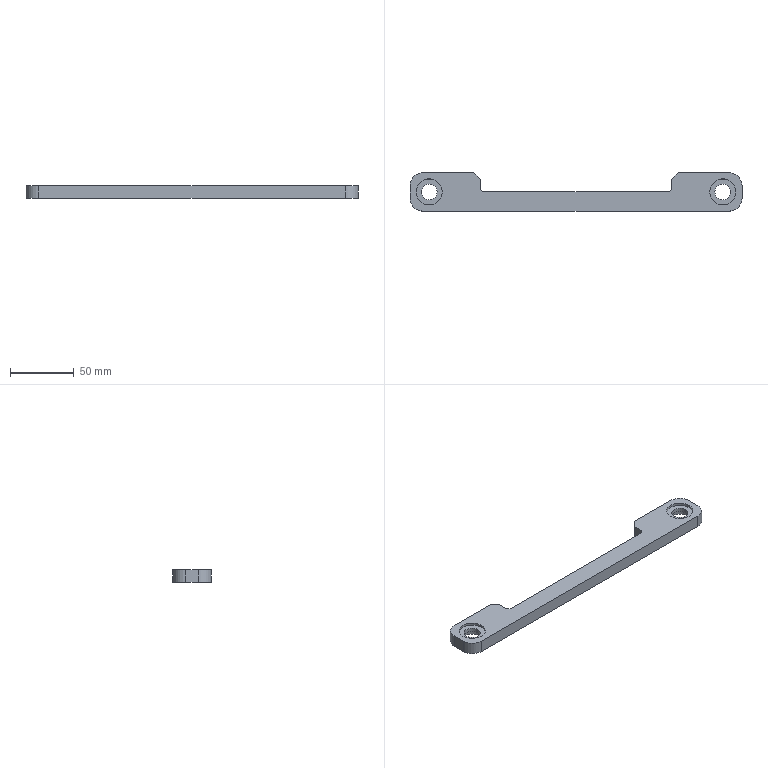Part | SolidWorks | features BaseBody 1 | 1 solid | 34 faces | box 260 x 30 x 10 mm | volume 49540 mm3 | plane 18 | cylinder 16 | commonest cylinder face diameters 12.5 x4 19 x4 20 x4 20.5 x4
STEP:
#1=CARTESIAN_POINT('',(-105.5,-44.517,281.481));
#2=VERTEX_POINT('',#1);
#3=CARTESIAN_POINT('',(-124.5,-44.517,281.481));
#4=VERTEX_POINT('',#3);
#5=CARTESIAN_POINT('',(-115.,-44.517,281.481));
#6=DIRECTION('',(0.,0.,-1.));
#7=DIRECTION('',(-1.,0.,0.));
#8=AXIS2_PLACEMENT_3D('',#5,#6,#7);
#9=CIRCLE('',#8,9.5);
#10=EDGE_CURVE('',#2,#4,#9,.T.);
#11=ORIENTED_EDGE('',*,*,#10,.F.);
#12=CARTESIAN_POINT('',(-105.5,-44.517,276.481));
#13=VERTEX_POINT('',#12);
#14=CARTESIAN_POINT('',(-105.5,-44.517,281.481));
#15=DIRECTION('',(0.,0.,-1.));
#16=VECTOR('',#15,1000.);
#17=LINE('',#14,#16);
#18=EDGE_CURVE('',#2,#13,#17,.T.);
#19=ORIENTED_EDGE('',*,*,#18,.T.);
#20=CARTESIAN_POINT('',(-124.5,-44.517,276.481));
#21=VERTEX_POINT('',#20);
#22=CARTESIAN_POINT('',(-115.,-44.517,276.481));
#23=DIRECTION('',(0.,0.,-1.));
#24=DIRECTION('',(-1.,0.,0.));
#25=AXIS2_PLACEMENT_3D('',#22,#23,#24);
#26=CIRCLE('',#25,9.5);
#27=EDGE_CURVE('',#13,#21,#26,.T.);
#28=ORIENTED_EDGE('',*,*,#27,.T.);
#29=CARTESIAN_POINT('',(-124.5,-44.517,281.481));
#30=DIRECTION('',(0.,0.,-1.));
#31=VECTOR('',#30,1000.);
#32=LINE('',#29,#31);
#33=EDGE_CURVE('',#4,#21,#32,.T.);
#34=ORIENTED_EDGE('',*,*,#33,.F.);
#35=EDGE_LOOP('',(#11,#19,#28,#34));
#36=FACE_OUTER_BOUND('',#35,.T.);
#37=CARTESIAN_POINT('',(-115.,-44.517,281.481));
#38=DIRECTION('',(0.,0.,-1.));
#39=DIRECTION('',(-1.,0.,0.));
#40=AXIS2_PLACEMENT_3D('',#37,#38,#39);
#41=CYLINDRICAL_SURFACE('',#40,9.5);
#42=ADVANCED_FACE('',(#36),#41,.F.);
#43=CARTESIAN_POINT('',(124.5,-44.517,281.481));
#44=VERTEX_POINT('',#43);
#45=CARTESIAN_POINT('',(105.5,-44.517,281.481));
#46=VERTEX_POINT('',#45);
#47=CARTESIAN_POINT('',(115.,-44.517,281.481));
#48=DIRECTION('',(0.,0.,-1.));
#49=DIRECTION('',(-1.,0.,0.));
#50=AXIS2_PLACEMENT_3D('',#47,#48,#49);
#51=CIRCLE('',#50,9.5);
#52=EDGE_CURVE('',#44,#46,#51,.T.);
#53=ORIENTED_EDGE('',*,*,#52,.F.);
#54=CARTESIAN_POINT('',(124.5,-44.517,276.481));
#55=VERTEX_POINT('',#54);
#56=CARTESIAN_POINT('',(124.5,-44.517,281.481));
#57=DIRECTION('',(0.,0.,-1.));
#58=VECTOR('',#57,1000.);
#59=LINE('',#56,#58);
#60=EDGE_CURVE('',#44,#55,#59,.T.);
#61=ORIENTED_EDGE('',*,*,#60,.T.);
#62=CARTESIAN_POINT('',(105.5,-44.517,276.481));
#63=VERTEX_POINT('',#62);
#64=CARTESIAN_POINT('',(115.,-44.517,276.481));
#65=DIRECTION('',(0.,0.,-1.));
#66=DIRECTION('',(-1.,0.,0.));
#67=AXIS2_PLACEMENT_3D('',#64,#65,#66);
#68=CIRCLE('',#67,9.5);
#69=EDGE_CURVE('',#55,#63,#68,.T.);
#70=ORIENTED_EDGE('',*,*,#69,.T.);
#71=CARTESIAN_POINT('',(105.5,-44.517,281.481));
#72=DIRECTION('',(0.,0.,-1.));
#73=VECTOR('',#72,1000.);
#74=LINE('',#71,#73);
#75=EDGE_CURVE('',#46,#63,#74,.T.);
#76=ORIENTED_EDGE('',*,*,#75,.F.);
#77=EDGE_LOOP('',(#53,#61,#70,#76));
#78=FACE_OUTER_BOUND('',#77,.T.);
#79=CARTESIAN_POINT('',(115.,-44.517,281.481));
#80=DIRECTION('',(0.,0.,-1.));
#81=DIRECTION('',(-1.,0.,0.));
#82=AXIS2_PLACEMENT_3D('',#79,#80,#81);
#83=CYLINDRICAL_SURFACE('',#82,9.5);
#84=ADVANCED_FACE('',(#78),#83,.F.);
#85=CARTESIAN_POINT('',(-125.25,-44.517,284.481));
#86=VERTEX_POINT('',#85);
#87=CARTESIAN_POINT('',(-104.75,-44.517,284.481));
#88=VERTEX_POINT('',#87);
#89=CARTESIAN_POINT('',(-115.,-44.517,284.481));
#90=DIRECTION('',(0.,0.,1.));
#91=DIRECTION('',(1.,0.,0.));
#92=AXIS2_PLACEMENT_3D('',#89,#90,#91);
#93=CIRCLE('',#92,10.25);
#94=EDGE_CURVE('',#86,#88,#93,.T.);
#95=ORIENTED_EDGE('',*,*,#94,.F.);
#96=CARTESIAN_POINT('',(-125.25,-44.517,286.481));
#97=VERTEX_POINT('',#96);
#98=CARTESIAN_POINT('',(-125.25,-44.517,284.481));
#99=DIRECTION('',(0.,0.,1.));
#100=VECTOR('',#99,1000.);
#101=LINE('',#98,#100);
#102=EDGE_CURVE('',#86,#97,#101,.T.);
#103=ORIENTED_EDGE('',*,*,#102,.T.);
#104=CARTESIAN_POINT('',(-104.75,-44.517,286.481));
#105=VERTEX_POINT('',#104);
#106=CARTESIAN_POINT('',(-115.,-44.517,286.481));
#107=DIRECTION('',(0.,0.,-1.));
#108=DIRECTION('',(1.,0.,0.));
#109=AXIS2_PLACEMENT_3D('',#106,#107,#108);
#110=CIRCLE('',#109,10.25);
#111=EDGE_CURVE('',#105,#97,#110,.T.);
#112=ORIENTED_EDGE('',*,*,#111,.F.);
#113=CARTESIAN_POINT('',(-104.75,-44.517,284.481));
#114=DIRECTION('',(0.,0.,1.));
#115=VECTOR('',#114,1000.);
#116=LINE('',#113,#115);
#117=EDGE_CURVE('',#88,#105,#116,.T.);
#118=ORIENTED_EDGE('',*,*,#117,.F.);
#119=EDGE_LOOP('',(#95,#103,#112,#118));
#120=FACE_OUTER_BOUND('',#119,.T.);
#121=CARTESIAN_POINT('',(-115.,-44.517,284.481));
#122=DIRECTION('',(0.,0.,1.));
#123=DIRECTION('',(1.,0.,0.));
#124=AXIS2_PLACEMENT_3D('',#121,#122,#123);
#125=CYLINDRICAL_SURFACE('',#124,10.25);
#126=ADVANCED_FACE('',(#120),#125,.F.);
#127=CARTESIAN_POINT('',(104.75,-44.517,284.481));
#128=VERTEX_POINT('',#127);
#129=CARTESIAN_POINT('',(125.25,-44.517,284.481));
#130=VERTEX_POINT('',#129);
#131=CARTESIAN_POINT('',(115.,-44.517,284.481));
#132=DIRECTION('',(0.,0.,1.));
#133=DIRECTION('',(1.,0.,0.));
#134=AXIS2_PLACEMENT_3D('',#131,#132,#133);
#135=CIRCLE('',#134,10.25);
#136=EDGE_CURVE('',#128,#130,#135,.T.);
#137=ORIENTED_EDGE('',*,*,#136,.F.);
#138=CARTESIAN_POINT('',(104.75,-44.517,286.481));
#139=VERTEX_POINT('',#138);
#140=CARTESIAN_POINT('',(104.75,-44.517,284.481));
#141=DIRECTION('',(0.,0.,1.));
#142=VECTOR('',#141,1000.);
#143=LINE('',#140,#142);
#144=EDGE_CURVE('',#128,#139,#143,.T.);
#145=ORIENTED_EDGE('',*,*,#144,.T.);
#146=CARTESIAN_POINT('',(125.25,-44.517,286.481));
#147=VERTEX_POINT('',#146);
#148=CARTESIAN_POINT('',(115.,-44.517,286.481));
#149=DIRECTION('',(0.,0.,-1.));
#150=DIRECTION('',(1.,0.,0.));
#151=AXIS2_PLACEMENT_3D('',#148,#149,#150);
#152=CIRCLE('',#151,10.25);
#153=EDGE_CURVE('',#147,#139,#152,.T.);
#154=ORIENTED_EDGE('',*,*,#153,.F.);
#155=CARTESIAN_POINT('',(125.25,-44.517,284.481));
#156=DIRECTION('',(0.,0.,1.));
#157=VECTOR('',#156,1000.);
#158=LINE('',#155,#157);
#159=EDGE_CURVE('',#130,#147,#158,.T.);
#160=ORIENTED_EDGE('',*,*,#159,.F.);
#161=EDGE_LOOP('',(#137,#145,#154,#160));
#162=FACE_OUTER_BOUND('',#161,.T.);
#163=CARTESIAN_POINT('',(115.,-44.517,284.481));
#164=DIRECTION('',(0.,0.,1.));
#165=DIRECTION('',(1.,0.,0.));
#166=AXIS2_PLACEMENT_3D('',#163,#164,#165);
#167=CYLINDRICAL_SURFACE('',#166,10.25);
#168=ADVANCED_FACE('',(#162),#167,.F.);
#169=CARTESIAN_POINT('',(-121.25,-44.517,281.481));
#170=VERTEX_POINT('',#169);
#171=CARTESIAN_POINT('',(-108.75,-44.517,281.481));
#172=VERTEX_POINT('',#171);
#173=CARTESIAN_POINT('',(-115.,-44.517,281.481));
#174=DIRECTION('',(0.,0.,1.));
#175=DIRECTION('',(1.,0.,0.));
#176=AXIS2_PLACEMENT_3D('',#173,#174,#175);
#177=CIRCLE('',#176,6.25);
#178=EDGE_CURVE('',#170,#172,#177,.T.);
#179=ORIENTED_EDGE('',*,*,#178,.F.);
#180=CARTESIAN_POINT('',(-121.25,-44.517,284.481));
#181=VERTEX_POINT('',#180);
#182=CARTESIAN_POINT('',(-121.25,-44.517,276.481));
#183=DIRECTION('',(0.,0.,1.));
#184=VECTOR('',#183,1000.);
#185=LINE('',#182,#184);
#186=EDGE_CURVE('',#170,#181,#185,.T.);
#187=ORIENTED_EDGE('',*,*,#186,.T.);
#188=CARTESIAN_POINT('',(-108.75,-44.517,284.481));
#189=VERTEX_POINT('',#188);
#190=CARTESIAN_POINT('',(-115.,-44.517,284.481));
#191=DIRECTION('',(0.,0.,-1.));
#192=DIRECTION('',(1.,0.,0.));
#193=AXIS2_PLACEMENT_3D('',#190,#191,#192);
#194=CIRCLE('',#193,6.25);
#195=EDGE_CURVE('',#189,#181,#194,.T.);
#196=ORIENTED_EDGE('',*,*,#195,.F.);
#197=CARTESIAN_POINT('',(-108.75,-44.517,276.481));
#198=DIRECTION('',(0.,0.,1.));
#199=VECTOR('',#198,1000.);
#200=LINE('',#197,#199);
#201=EDGE_CURVE('',#172,#189,#200,.T.);
#202=ORIENTED_EDGE('',*,*,#201,.F.);
#203=EDGE_LOOP('',(#179,#187,#196,#202));
#204=FACE_OUTER_BOUND('',#203,.T.);
#205=CARTESIAN_POINT('',(-115.,-44.517,276.481));
#206=DIRECTION('',(0.,0.,1.));
#207=DIRECTION('',(1.,0.,0.));
#208=AXIS2_PLACEMENT_3D('',#205,#206,#207);
#209=CYLINDRICAL_SURFACE('',#208,6.25);
#210=ADVANCED_FACE('',(#204),#209,.F.);
#211=CARTESIAN_POINT('',(108.75,-44.517,281.481));
#212=VERTEX_POINT('',#211);
#213=CARTESIAN_POINT('',(121.25,-44.517,281.481));
#214=VERTEX_POINT('',#213);
#215=CARTESIAN_POINT('',(115.,-44.517,281.481));
#216=DIRECTION('',(0.,0.,1.));
#217=DIRECTION('',(1.,0.,0.));
#218=AXIS2_PLACEMENT_3D('',#215,#216,#217);
#219=CIRCLE('',#218,6.25);
#220=EDGE_CURVE('',#212,#214,#219,.T.);
#221=ORIENTED_EDGE('',*,*,#220,.F.);
#222=CARTESIAN_POINT('',(108.75,-44.517,284.481));
#223=VERTEX_POINT('',#222);
#224=CARTESIAN_POINT('',(108.75,-44.517,276.481));
#225=DIRECTION('',(0.,0.,1.));
#226=VECTOR('',#225,1000.);
#227=LINE('',#224,#226);
#228=EDGE_CURVE('',#212,#223,#227,.T.);
#229=ORIENTED_EDGE('',*,*,#228,.T.);
#230=CARTESIAN_POINT('',(121.25,-44.517,284.481));
#231=VERTEX_POINT('',#230);
#232=CARTESIAN_POINT('',(115.,-44.517,284.481));
#233=DIRECTION('',(0.,0.,-1.));
#234=DIRECTION('',(1.,0.,0.));
#235=AXIS2_PLACEMENT_3D('',#232,#233,#234);
#236=CIRCLE('',#235,6.25);
#237=EDGE_CURVE('',#231,#223,#236,.T.);
#238=ORIENTED_EDGE('',*,*,#237,.F.);
#239=CARTESIAN_POINT('',(121.25,-44.517,276.481));
#240=DIRECTION('',(0.,0.,1.));
#241=VECTOR('',#240,1000.);
#242=LINE('',#239,#241);
#243=EDGE_CURVE('',#214,#231,#242,.T.);
#244=ORIENTED_EDGE('',*,*,#243,.F.);
#245=EDGE_LOOP('',(#221,#229,#238,#244));
#246=FACE_OUTER_BOUND('',#245,.T.);
#247=CARTESIAN_POINT('',(115.,-44.517,276.481));
#248=DIRECTION('',(0.,0.,1.));
#249=DIRECTION('',(1.,0.,0.));
#250=AXIS2_PLACEMENT_3D('',#247,#248,#249);
#251=CYLINDRICAL_SURFACE('',#250,6.25);
#252=ADVANCED_FACE('',(#246),#251,.F.);
#253=CARTESIAN_POINT('',(-75.,-34.517,276.481));
#254=VERTEX_POINT('',#253);
#255=CARTESIAN_POINT('',(-80.,-29.517,276.481));
#256=VERTEX_POINT('',#255);
#257=CARTESIAN_POINT('',(-75.,-34.517,276.481));
#258=DIRECTION('',(-0.7071,0.7071,0.));
#259=VECTOR('',#258,1000.);
#260=LINE('',#257,#259);
#261=EDGE_CURVE('',#254,#256,#260,.T.);
#262=ORIENTED_EDGE('',*,*,#261,.F.);
#263=CARTESIAN_POINT('',(-75.,-42.517,276.481));
#264=VERTEX_POINT('',#263);
#265=CARTESIAN_POINT('',(-75.,-44.517,276.481));
#266=DIRECTION('',(0.,1.,0.));
#267=VECTOR('',#266,1000.);
#268=LINE('',#265,#267);
#269=EDGE_CURVE('',#264,#254,#268,.T.);
#270=ORIENTED_EDGE('',*,*,#269,.F.);
#271=CARTESIAN_POINT('',(-73.,-44.517,276.481));
#272=VERTEX_POINT('',#271);
#273=CARTESIAN_POINT('',(-73.,-44.517,276.481));
#274=DIRECTION('',(-0.7071,0.7071,0.));
#275=VECTOR('',#274,1000.);
#276=LINE('',#273,#275);
#277=EDGE_CURVE('',#272,#264,#276,.T.);
#278=ORIENTED_EDGE('',*,*,#277,.F.);
#279=CARTESIAN_POINT('',(73.,-44.517,276.481));
#280=VERTEX_POINT('',#279);
#281=CARTESIAN_POINT('',(0.,-44.517,276.481));
#282=DIRECTION('',(-1.,0.,0.));
#283=VECTOR('',#282,1000.);
#284=LINE('',#281,#283);
#285=EDGE_CURVE('',#280,#272,#284,.T.);
#286=ORIENTED_EDGE('',*,*,#285,.F.);
#287=CARTESIAN_POINT('',(75.,-42.517,276.481));
#288=VERTEX_POINT('',#287);
#289=CARTESIAN_POINT('',(75.,-42.517,276.481));
#290=DIRECTION('',(-0.7071,-0.7071,0.));
#291=VECTOR('',#290,1000.);
#292=LINE('',#289,#291);
#293=EDGE_CURVE('',#288,#280,#292,.T.);
#294=ORIENTED_EDGE('',*,*,#293,.F.);
#295=CARTESIAN_POINT('',(75.,-34.517,276.481));
#296=VERTEX_POINT('',#295);
#297=CARTESIAN_POINT('',(75.,-44.517,276.481));
#298=DIRECTION('',(0.,-1.,0.));
#299=VECTOR('',#298,1000.);
#300=LINE('',#297,#299);
#301=EDGE_CURVE('',#296,#288,#300,.T.);
#302=ORIENTED_EDGE('',*,*,#301,.F.);
#303=CARTESIAN_POINT('',(80.,-29.517,276.481));
#304=VERTEX_POINT('',#303);
#305=CARTESIAN_POINT('',(80.,-29.517,276.481));
#306=DIRECTION('',(-0.7071,-0.7071,0.));
#307=VECTOR('',#306,1000.);
#308=LINE('',#305,#307);
#309=EDGE_CURVE('',#304,#296,#308,.T.);
#310=ORIENTED_EDGE('',*,*,#309,.F.);
#311=CARTESIAN_POINT('',(120.,-29.517,276.481));
#312=VERTEX_POINT('',#311);
#313=CARTESIAN_POINT('',(0.,-29.517,276.481));
#314=DIRECTION('',(-1.,0.,0.));
#315=VECTOR('',#314,1000.);
#316=LINE('',#313,#315);
#317=EDGE_CURVE('',#312,#304,#316,.T.);
#318=ORIENTED_EDGE('',*,*,#317,.F.);
#319=CARTESIAN_POINT('',(130.,-39.517,276.481));
#320=VERTEX_POINT('',#319);
#321=CARTESIAN_POINT('',(120.,-39.517,276.481));
#322=DIRECTION('',(0.,0.,1.));
#323=DIRECTION('',(-1.,0.,0.));
#324=AXIS2_PLACEMENT_3D('',#321,#322,#323);
#325=CIRCLE('',#324,10.);
#326=EDGE_CURVE('',#320,#312,#325,.T.);
#327=ORIENTED_EDGE('',*,*,#326,.F.);
#328=CARTESIAN_POINT('',(130.,-49.517,276.481));
#329=VERTEX_POINT('',#328);
#330=CARTESIAN_POINT('',(130.,-44.517,276.481));
#331=DIRECTION('',(0.,1.,0.));
#332=VECTOR('',#331,1000.);
#333=LINE('',#330,#332);
#334=EDGE_CURVE('',#329,#320,#333,.T.);
#335=ORIENTED_EDGE('',*,*,#334,.F.);
#336=CARTESIAN_POINT('',(120.,-59.517,276.481));
#337=VERTEX_POINT('',#336);
#338=CARTESIAN_POINT('',(120.,-49.517,276.481));
#339=DIRECTION('',(0.,0.,1.));
#340=DIRECTION('',(-1.,0.,0.));
#341=AXIS2_PLACEMENT_3D('',#338,#339,#340);
#342=CIRCLE('',#341,10.);
#343=EDGE_CURVE('',#337,#329,#342,.T.);
#344=ORIENTED_EDGE('',*,*,#343,.F.);
#345=CARTESIAN_POINT('',(-120.,-59.517,276.481));
#346=VERTEX_POINT('',#345);
#347=CARTESIAN_POINT('',(0.,-59.517,276.481));
#348=DIRECTION('',(1.,0.,0.));
#349=VECTOR('',#348,1000.);
#350=LINE('',#347,#349);
#351=EDGE_CURVE('',#346,#337,#350,.T.);
#352=ORIENTED_EDGE('',*,*,#351,.F.);
#353=CARTESIAN_POINT('',(-130.,-49.517,276.481));
#354=VERTEX_POINT('',#353);
#355=CARTESIAN_POINT('',(-120.,-49.517,276.481));
#356=DIRECTION('',(0.,0.,1.));
#357=DIRECTION('',(-1.,0.,0.));
#358=AXIS2_PLACEMENT_3D('',#355,#356,#357);
#359=CIRCLE('',#358,10.);
#360=EDGE_CURVE('',#354,#346,#359,.T.);
#361=ORIENTED_EDGE('',*,*,#360,.F.);
#362=CARTESIAN_POINT('',(-130.,-39.517,276.481));
#363=VERTEX_POINT('',#362);
#364=CARTESIAN_POINT('',(-130.,-44.517,276.481));
#365=DIRECTION('',(0.,-1.,0.));
#366=VECTOR('',#365,1000.);
#367=LINE('',#364,#366);
#368=EDGE_CURVE('',#363,#354,#367,.T.);
#369=ORIENTED_EDGE('',*,*,#368,.F.);
#370=CARTESIAN_POINT('',(-120.,-29.517,276.481));
#371=VERTEX_POINT('',#370);
#372=CARTESIAN_POINT('',(-120.,-39.517,276.481));
#373=DIRECTION('',(0.,0.,1.));
#374=DIRECTION('',(-1.,0.,0.));
#375=AXIS2_PLACEMENT_3D('',#372,#373,#374);
#376=CIRCLE('',#375,10.);
#377=EDGE_CURVE('',#371,#363,#376,.T.);
#378=ORIENTED_EDGE('',*,*,#377,.F.);
#379=CARTESIAN_POINT('',(0.,-29.517,276.481));
#380=DIRECTION('',(-1.,0.,0.));
#381=VECTOR('',#380,1000.);
#382=LINE('',#379,#381);
#383=EDGE_CURVE('',#256,#371,#382,.T.);
#384=ORIENTED_EDGE('',*,*,#383,.F.);
#385=EDGE_LOOP('',(#262,#270,#278,#286,#294,#302,#310,#318,#327,#335,#344,#352,#361,#369,#378,#384));
#386=FACE_OUTER_BOUND('',#385,.T.);
#387=CARTESIAN_POINT('',(-115.,-44.517,276.481));
#388=DIRECTION('',(0.,0.,-1.));
#389=DIRECTION('',(-1.,0.,0.));
#390=AXIS2_PLACEMENT_3D('',#387,#388,#389);
#391=CIRCLE('',#390,9.5);
#392=EDGE_CURVE('',#21,#13,#391,.T.);
#393=ORIENTED_EDGE('',*,*,#392,.F.);
#394=ORIENTED_EDGE('',*,*,#27,.F.);
#395=EDGE_LOOP('',(#393,#394));
#396=FACE_BOUND('',#395,.T.);
#397=CARTESIAN_POINT('',(115.,-44.517,276.481));
#398=DIRECTION('',(0.,0.,-1.));
#399=DIRECTION('',(-1.,0.,0.));
#400=AXIS2_PLACEMENT_3D('',#397,#398,#399);
#401=CIRCLE('',#400,9.5);
#402=EDGE_CURVE('',#63,#55,#401,.T.);
#403=ORIENTED_EDGE('',*,*,#402,.F.);
#404=ORIENTED_EDGE('',*,*,#69,.F.);
#405=EDGE_LOOP('',(#403,#404));
#406=FACE_BOUND('',#405,.T.);
#407=CARTESIAN_POINT('',(0.,-44.517,276.481));
#408=DIRECTION('',(0.,0.,1.));
#409=DIRECTION('',(1.,0.,0.));
#410=AXIS2_PLACEMENT_3D('',#407,#408,#409);
#411=PLANE('',#410);
#412=ADVANCED_FACE('',(#386,#396,#406),#411,.F.);
#413=CARTESIAN_POINT('',(-80.,-29.517,286.481));
#414=VERTEX_POINT('',#413);
#415=CARTESIAN_POINT('',(-80.,-29.517,286.481));
#416=DIRECTION('',(0.,0.,1.));
#417=VECTOR('',#416,1000.);
#418=LINE('',#415,#417);
#419=EDGE_CURVE('',#256,#414,#418,.T.);
#420=ORIENTED_EDGE('',*,*,#419,.F.);
#421=ORIENTED_EDGE('',*,*,#383,.T.);
#422=CARTESIAN_POINT('',(-120.,-29.517,286.481));
#423=VERTEX_POINT('',#422);
#424=CARTESIAN_POINT('',(-120.,-29.517,286.481));
#425=DIRECTION('',(0.,0.,-1.));
#426=VECTOR('',#425,1000.);
#427=LINE('',#424,#426);
#428=EDGE_CURVE('',#423,#371,#427,.T.);
#429=ORIENTED_EDGE('',*,*,#428,.F.);
#430=CARTESIAN_POINT('',(130.,-29.517,286.481));
#431=DIRECTION('',(-1.,0.,0.));
#432=VECTOR('',#431,1000.);
#433=LINE('',#430,#432);
#434=EDGE_CURVE('',#414,#423,#433,.T.);
#435=ORIENTED_EDGE('',*,*,#434,.F.);
#436=EDGE_LOOP('',(#420,#421,#429,#435));
#437=FACE_OUTER_BOUND('',#436,.T.);
#438=CARTESIAN_POINT('',(130.,-29.517,286.481));
#439=DIRECTION('',(0.,-1.,0.));
#440=DIRECTION('',(0.,0.,-1.));
#441=AXIS2_PLACEMENT_3D('',#438,#439,#440);
#442=PLANE('',#441);
#443=ADVANCED_FACE('',(#437),#442,.F.);
#444=CARTESIAN_POINT('',(-75.,-34.517,286.481));
#445=VERTEX_POINT('',#444);
#446=CARTESIAN_POINT('',(-75.,-34.517,286.481));
#447=DIRECTION('',(0.,0.,1.));
#448=VECTOR('',#447,1000.);
#449=LINE('',#446,#448);
#450=EDGE_CURVE('',#254,#445,#449,.T.);
#451=ORIENTED_EDGE('',*,*,#450,.F.);
#452=ORIENTED_EDGE('',*,*,#261,.T.);
#453=ORIENTED_EDGE('',*,*,#419,.T.);
#454=CARTESIAN_POINT('',(-80.,-29.517,286.481));
#455=DIRECTION('',(-0.7071,0.7071,0.));
#456=VECTOR('',#455,1000.);
#457=LINE('',#454,#456);
#458=EDGE_CURVE('',#445,#414,#457,.T.);
#459=ORIENTED_EDGE('',*,*,#458,.F.);
#460=EDGE_LOOP('',(#451,#452,#453,#459));
#461=FACE_OUTER_BOUND('',#460,.T.);
#462=CARTESIAN_POINT('',(-80.,-29.517,286.481));
#463=DIRECTION('',(-0.7071,-0.7071,0.));
#464=DIRECTION('',(0.7071,-0.7071,0.));
#465=AXIS2_PLACEMENT_3D('',#462,#463,#464);
#466=PLANE('',#465);
#467=ADVANCED_FACE('',(#461),#466,.F.);
#468=ORIENTED_EDGE('',*,*,#450,.T.);
#469=CARTESIAN_POINT('',(-75.,-42.517,286.481));
#470=VERTEX_POINT('',#469);
#471=CARTESIAN_POINT('',(-75.,-14.517,286.481));
#472=DIRECTION('',(0.,1.,0.));
#473=VECTOR('',#472,1000.);
#474=LINE('',#471,#473);
#475=EDGE_CURVE('',#470,#445,#474,.T.);
#476=ORIENTED_EDGE('',*,*,#475,.F.);
#477=CARTESIAN_POINT('',(-75.,-42.517,286.481));
#478=DIRECTION('',(0.,0.,1.));
#479=VECTOR('',#478,1000.);
#480=LINE('',#477,#479);
#481=EDGE_CURVE('',#264,#470,#480,.T.);
#482=ORIENTED_EDGE('',*,*,#481,.F.);
#483=ORIENTED_EDGE('',*,*,#269,.T.);
#484=EDGE_LOOP('',(#468,#476,#482,#483));
#485=FACE_OUTER_BOUND('',#484,.T.);
#486=CARTESIAN_POINT('',(-75.,-14.517,286.481));
#487=DIRECTION('',(-1.,0.,0.));
#488=DIRECTION('',(0.,0.,1.));
#489=AXIS2_PLACEMENT_3D('',#486,#487,#488);
#490=PLANE('',#489);
#491=ADVANCED_FACE('',(#485),#490,.F.);
#492=ORIENTED_EDGE('',*,*,#277,.T.);
#493=ORIENTED_EDGE('',*,*,#481,.T.);
#494=CARTESIAN_POINT('',(-73.,-44.517,286.481));
#495=VERTEX_POINT('',#494);
#496=CARTESIAN_POINT('',(-75.,-42.517,286.481));
#497=DIRECTION('',(0.7071,-0.7071,0.));
#498=VECTOR('',#497,1000.);
#499=LINE('',#496,#498);
#500=EDGE_CURVE('',#470,#495,#499,.T.);
#501=ORIENTED_EDGE('',*,*,#500,.T.);
#502=CARTESIAN_POINT('',(-73.,-44.517,286.481));
#503=DIRECTION('',(0.,0.,-1.));
#504=VECTOR('',#503,1000.);
#505=LINE('',#502,#504);
#506=EDGE_CURVE('',#495,#272,#505,.T.);
#507=ORIENTED_EDGE('',*,*,#506,.T.);
#508=EDGE_LOOP('',(#492,#493,#501,#507));
#509=FACE_OUTER_BOUND('',#508,.T.);
#510=CARTESIAN_POINT('',(-75.,-42.517,286.481));
#511=DIRECTION('',(0.7071,0.7071,0.));
#512=DIRECTION('',(-0.7071,0.7071,0.));
#513=AXIS2_PLACEMENT_3D('',#510,#511,#512);
#514=PLANE('',#513);
#515=ADVANCED_FACE('',(#509),#514,.T.);
#516=ORIENTED_EDGE('',*,*,#506,.F.);
#517=CARTESIAN_POINT('',(73.,-44.517,286.481));
#518=VERTEX_POINT('',#517);
#519=CARTESIAN_POINT('',(75.,-44.517,286.481));
#520=DIRECTION('',(-1.,0.,0.));
#521=VECTOR('',#520,1000.);
#522=LINE('',#519,#521);
#523=EDGE_CURVE('',#518,#495,#522,.T.);
#524=ORIENTED_EDGE('',*,*,#523,.F.);
#525=CARTESIAN_POINT('',(73.,-44.517,286.481));
#526=DIRECTION('',(0.,0.,1.));
#527=VECTOR('',#526,1000.);
#528=LINE('',#525,#527);
#529=EDGE_CURVE('',#280,#518,#528,.T.);
#530=ORIENTED_EDGE('',*,*,#529,.F.);
#531=ORIENTED_EDGE('',*,*,#285,.T.);
#532=EDGE_LOOP('',(#516,#524,#530,#531));
#533=FACE_OUTER_BOUND('',#532,.T.);
#534=CARTESIAN_POINT('',(75.,-44.517,286.481));
#535=DIRECTION('',(0.,-1.,0.));
#536=DIRECTION('',(0.,0.,-1.));
#537=AXIS2_PLACEMENT_3D('',#534,#535,#536);
#538=PLANE('',#537);
#539=ADVANCED_FACE('',(#533),#538,.F.);
#540=ORIENTED_EDGE('',*,*,#293,.T.);
#541=ORIENTED_EDGE('',*,*,#529,.T.);
#542=CARTESIAN_POINT('',(75.,-42.517,286.481));
#543=VERTEX_POINT('',#542);
#544=CARTESIAN_POINT('',(73.,-44.517,286.481));
#545=DIRECTION('',(0.7071,0.7071,0.));
#546=VECTOR('',#545,1000.);
#547=LINE('',#544,#546);
#548=EDGE_CURVE('',#518,#543,#547,.T.);
#549=ORIENTED_EDGE('',*,*,#548,.T.);
#550=CARTESIAN_POINT('',(75.,-42.517,286.481));
#551=DIRECTION('',(0.,0.,-1.));
#552=VECTOR('',#551,1000.);
#553=LINE('',#550,#552);
#554=EDGE_CURVE('',#543,#288,#553,.T.);
#555=ORIENTED_EDGE('',*,*,#554,.T.);
#556=EDGE_LOOP('',(#540,#541,#549,#555));
#557=FACE_OUTER_BOUND('',#556,.T.);
#558=CARTESIAN_POINT('',(73.,-44.517,286.481));
#559=DIRECTION('',(-0.7071,0.7071,0.));
#560=DIRECTION('',(-0.7071,-0.7071,0.));
#561=AXIS2_PLACEMENT_3D('',#558,#559,#560);
#562=PLANE('',#561);
#563=ADVANCED_FACE('',(#557),#562,.T.);
#564=CARTESIAN_POINT('',(75.,-34.517,286.481));
#565=VERTEX_POINT('',#564);
#566=CARTESIAN_POINT('',(75.,-34.517,286.481));
#567=DIRECTION('',(0.,0.,1.));
#568=VECTOR('',#567,1000.);
#569=LINE('',#566,#568);
#570=EDGE_CURVE('',#296,#565,#569,.T.);
#571=ORIENTED_EDGE('',*,*,#570,.F.);
#572=ORIENTED_EDGE('',*,*,#301,.T.);
#573=ORIENTED_EDGE('',*,*,#554,.F.);
#574=CARTESIAN_POINT('',(75.,-14.517,286.481));
#575=DIRECTION('',(0.,-1.,0.));
#576=VECTOR('',#575,1000.);
#577=LINE('',#574,#576);
#578=EDGE_CURVE('',#565,#543,#577,.T.);
#579=ORIENTED_EDGE('',*,*,#578,.F.);
#580=EDGE_LOOP('',(#571,#572,#573,#579));
#581=FACE_OUTER_BOUND('',#580,.T.);
#582=CARTESIAN_POINT('',(75.,-14.517,286.481));
#583=DIRECTION('',(1.,0.,0.));
#584=DIRECTION('',(0.,0.,-1.));
#585=AXIS2_PLACEMENT_3D('',#582,#583,#584);
#586=PLANE('',#585);
#587=ADVANCED_FACE('',(#581),#586,.F.);
#588=ORIENTED_EDGE('',*,*,#570,.T.);
#589=CARTESIAN_POINT('',(80.,-29.517,286.481));
#590=VERTEX_POINT('',#589);
#591=CARTESIAN_POINT('',(80.,-29.517,286.481));
#592=DIRECTION('',(-0.7071,-0.7071,0.));
#593=VECTOR('',#592,1000.);
#594=LINE('',#591,#593);
#595=EDGE_CURVE('',#590,#565,#594,.T.);
#596=ORIENTED_EDGE('',*,*,#595,.F.);
#597=CARTESIAN_POINT('',(80.,-29.517,286.481));
#598=DIRECTION('',(0.,0.,1.));
#599=VECTOR('',#598,1000.);
#600=LINE('',#597,#599);
#601=EDGE_CURVE('',#304,#590,#600,.T.);
#602=ORIENTED_EDGE('',*,*,#601,.F.);
#603=ORIENTED_EDGE('',*,*,#309,.T.);
#604=EDGE_LOOP('',(#588,#596,#602,#603));
#605=FACE_OUTER_BOUND('',#604,.T.);
#606=CARTESIAN_POINT('',(80.,-29.517,286.481));
#607=DIRECTION('',(0.7071,-0.7071,0.));
#608=DIRECTION('',(0.7071,0.7071,0.));
#609=AXIS2_PLACEMENT_3D('',#606,#607,#608);
#610=PLANE('',#609);
#611=ADVANCED_FACE('',(#605),#610,.F.);
#612=ORIENTED_EDGE('',*,*,#601,.T.);
#613=CARTESIAN_POINT('',(120.,-29.517,286.481));
#614=VERTEX_POINT('',#613);
#615=CARTESIAN_POINT('',(130.,-29.517,286.481));
#616=DIRECTION('',(-1.,0.,0.));
#617=VECTOR('',#616,1000.);
#618=LINE('',#615,#617);
#619=EDGE_CURVE('',#614,#590,#618,.T.);
#620=ORIENTED_EDGE('',*,*,#619,.F.);
#621=CARTESIAN_POINT('',(120.,-29.517,286.481));
#622=DIRECTION('',(0.,0.,1.));
#623=VECTOR('',#622,1000.);
#624=LINE('',#621,#623);
#625=EDGE_CURVE('',#312,#614,#624,.T.);
#626=ORIENTED_EDGE('',*,*,#625,.F.);
#627=ORIENTED_EDGE('',*,*,#317,.T.);
#628=EDGE_LOOP('',(#612,#620,#626,#627));
#629=FACE_OUTER_BOUND('',#628,.T.);
#630=CARTESIAN_POINT('',(130.,-29.517,286.481));
#631=DIRECTION('',(0.,-1.,0.));
#632=DIRECTION('',(0.,0.,-1.));
#633=AXIS2_PLACEMENT_3D('',#630,#631,#632);
#634=PLANE('',#633);
#635=ADVANCED_FACE('',(#629),#634,.F.);
#636=ORIENTED_EDGE('',*,*,#326,.T.);
#637=ORIENTED_EDGE('',*,*,#625,.T.);
#638=CARTESIAN_POINT('',(130.,-39.517,286.481));
#639=VERTEX_POINT('',#638);
#640=CARTESIAN_POINT('',(120.,-39.517,286.481));
#641=DIRECTION('',(0.,0.,-1.));
#642=DIRECTION('',(-1.,0.,0.));
#643=AXIS2_PLACEMENT_3D('',#640,#641,#642);
#644=CIRCLE('',#643,10.);
#645=EDGE_CURVE('',#614,#639,#644,.T.);
#646=ORIENTED_EDGE('',*,*,#645,.T.);
#647=CARTESIAN_POINT('',(130.,-39.517,286.481));
#648=DIRECTION('',(0.,0.,-1.));
#649=VECTOR('',#648,1000.);
#650=LINE('',#647,#649);
#651=EDGE_CURVE('',#639,#320,#650,.T.);
#652=ORIENTED_EDGE('',*,*,#651,.T.);
#653=EDGE_LOOP('',(#636,#637,#646,#652));
#654=FACE_OUTER_BOUND('',#653,.T.);
#655=CARTESIAN_POINT('',(120.,-39.517,286.481));
#656=DIRECTION('',(0.,0.,-1.));
#657=DIRECTION('',(-1.,0.,0.));
#658=AXIS2_PLACEMENT_3D('',#655,#656,#657);
#659=CYLINDRICAL_SURFACE('',#658,10.);
#660=ADVANCED_FACE('',(#654),#659,.T.);
#661=ORIENTED_EDGE('',*,*,#651,.F.);
#662=CARTESIAN_POINT('',(130.,-49.517,286.481));
#663=VERTEX_POINT('',#662);
#664=CARTESIAN_POINT('',(130.,-59.517,286.481));
#665=DIRECTION('',(0.,1.,0.));
#666=VECTOR('',#665,1000.);
#667=LINE('',#664,#666);
#668=EDGE_CURVE('',#663,#639,#667,.T.);
#669=ORIENTED_EDGE('',*,*,#668,.F.);
#670=CARTESIAN_POINT('',(130.,-49.517,286.481));
#671=DIRECTION('',(0.,0.,1.));
#672=VECTOR('',#671,1000.);
#673=LINE('',#670,#672);
#674=EDGE_CURVE('',#329,#663,#673,.T.);
#675=ORIENTED_EDGE('',*,*,#674,.F.);
#676=ORIENTED_EDGE('',*,*,#334,.T.);
#677=EDGE_LOOP('',(#661,#669,#675,#676));
#678=FACE_OUTER_BOUND('',#677,.T.);
#679=CARTESIAN_POINT('',(130.,-59.517,286.481));
#680=DIRECTION('',(-1.,0.,0.));
#681=DIRECTION('',(0.,0.,1.));
#682=AXIS2_PLACEMENT_3D('',#679,#680,#681);
#683=PLANE('',#682);
#684=ADVANCED_FACE('',(#678),#683,.F.);
#685=ORIENTED_EDGE('',*,*,#343,.T.);
#686=ORIENTED_EDGE('',*,*,#674,.T.);
#687=CARTESIAN_POINT('',(120.,-59.517,286.481));
#688=VERTEX_POINT('',#687);
#689=CARTESIAN_POINT('',(120.,-49.517,286.481));
#690=DIRECTION('',(0.,0.,-1.));
#691=DIRECTION('',(-1.,0.,0.));
#692=AXIS2_PLACEMENT_3D('',#689,#690,#691);
#693=CIRCLE('',#692,10.);
#694=EDGE_CURVE('',#663,#688,#693,.T.);
#695=ORIENTED_EDGE('',*,*,#694,.T.);
#696=CARTESIAN_POINT('',(120.,-59.517,286.481));
#697=DIRECTION('',(0.,0.,-1.));
#698=VECTOR('',#697,1000.);
#699=LINE('',#696,#698);
#700=EDGE_CURVE('',#688,#337,#699,.T.);
#701=ORIENTED_EDGE('',*,*,#700,.T.);
#702=EDGE_LOOP('',(#685,#686,#695,#701));
#703=FACE_OUTER_BOUND('',#702,.T.);
#704=CARTESIAN_POINT('',(120.,-49.517,286.481));
#705=DIRECTION('',(0.,0.,-1.));
#706=DIRECTION('',(-1.,0.,0.));
#707=AXIS2_PLACEMENT_3D('',#704,#705,#706);
#708=CYLINDRICAL_SURFACE('',#707,10.);
#709=ADVANCED_FACE('',(#703),#708,.T.);
#710=ORIENTED_EDGE('',*,*,#700,.F.);
#711=CARTESIAN_POINT('',(-120.,-59.517,286.481));
#712=VERTEX_POINT('',#711);
#713=CARTESIAN_POINT('',(130.,-59.517,286.481));
#714=DIRECTION('',(1.,0.,0.));
#715=VECTOR('',#714,1000.);
#716=LINE('',#713,#715);
#717=EDGE_CURVE('',#712,#688,#716,.T.);
#718=ORIENTED_EDGE('',*,*,#717,.F.);
#719=CARTESIAN_POINT('',(-120.,-59.517,286.481));
#720=DIRECTION('',(0.,0.,1.));
#721=VECTOR('',#720,1000.);
#722=LINE('',#719,#721);
#723=EDGE_CURVE('',#346,#712,#722,.T.);
#724=ORIENTED_EDGE('',*,*,#723,.F.);
#725=ORIENTED_EDGE('',*,*,#351,.T.);
#726=EDGE_LOOP('',(#710,#718,#724,#725));
#727=FACE_OUTER_BOUND('',#726,.T.);
#728=CARTESIAN_POINT('',(130.,-59.517,286.481));
#729=DIRECTION('',(0.,1.,0.));
#730=DIRECTION('',(0.,0.,1.));
#731=AXIS2_PLACEMENT_3D('',#728,#729,#730);
#732=PLANE('',#731);
#733=ADVANCED_FACE('',(#727),#732,.F.);
#734=ORIENTED_EDGE('',*,*,#360,.T.);
#735=ORIENTED_EDGE('',*,*,#723,.T.);
#736=CARTESIAN_POINT('',(-130.,-49.517,286.481));
#737=VERTEX_POINT('',#736);
#738=CARTESIAN_POINT('',(-120.,-49.517,286.481));
#739=DIRECTION('',(0.,0.,-1.));
#740=DIRECTION('',(-1.,0.,0.));
#741=AXIS2_PLACEMENT_3D('',#738,#739,#740);
#742=CIRCLE('',#741,10.);
#743=EDGE_CURVE('',#712,#737,#742,.T.);
#744=ORIENTED_EDGE('',*,*,#743,.T.);
#745=CARTESIAN_POINT('',(-130.,-49.517,286.481));
#746=DIRECTION('',(0.,0.,-1.));
#747=VECTOR('',#746,1000.);
#748=LINE('',#745,#747);
#749=EDGE_CURVE('',#737,#354,#748,.T.);
#750=ORIENTED_EDGE('',*,*,#749,.T.);
#751=EDGE_LOOP('',(#734,#735,#744,#750));
#752=FACE_OUTER_BOUND('',#751,.T.);
#753=CARTESIAN_POINT('',(-120.,-49.517,286.481));
#754=DIRECTION('',(0.,0.,-1.));
#755=DIRECTION('',(-1.,0.,0.));
#756=AXIS2_PLACEMENT_3D('',#753,#754,#755);
#757=CYLINDRICAL_SURFACE('',#756,10.);
#758=ADVANCED_FACE('',(#752),#757,.T.);
#759=CARTESIAN_POINT('',(-130.,-39.517,286.481));
#760=VERTEX_POINT('',#759);
#761=CARTESIAN_POINT('',(-130.,-39.517,286.481));
#762=DIRECTION('',(0.,0.,1.));
#763=VECTOR('',#762,1000.);
#764=LINE('',#761,#763);
#765=EDGE_CURVE('',#363,#760,#764,.T.);
#766=ORIENTED_EDGE('',*,*,#765,.F.);
#767=ORIENTED_EDGE('',*,*,#368,.T.);
#768=ORIENTED_EDGE('',*,*,#749,.F.);
#769=CARTESIAN_POINT('',(-130.,-59.517,286.481));
#770=DIRECTION('',(0.,-1.,0.));
#771=VECTOR('',#770,1000.);
#772=LINE('',#769,#771);
#773=EDGE_CURVE('',#760,#737,#772,.T.);
#774=ORIENTED_EDGE('',*,*,#773,.F.);
#775=EDGE_LOOP('',(#766,#767,#768,#774));
#776=FACE_OUTER_BOUND('',#775,.T.);
#777=CARTESIAN_POINT('',(-130.,-59.517,286.481));
#778=DIRECTION('',(1.,0.,0.));
#779=DIRECTION('',(0.,0.,-1.));
#780=AXIS2_PLACEMENT_3D('',#777,#778,#779);
#781=PLANE('',#780);
#782=ADVANCED_FACE('',(#776),#781,.F.);
#783=ORIENTED_EDGE('',*,*,#377,.T.);
#784=ORIENTED_EDGE('',*,*,#765,.T.);
#785=CARTESIAN_POINT('',(-120.,-39.517,286.481));
#786=DIRECTION('',(0.,0.,-1.));
#787=DIRECTION('',(-1.,0.,0.));
#788=AXIS2_PLACEMENT_3D('',#785,#786,#787);
#789=CIRCLE('',#788,10.);
#790=EDGE_CURVE('',#760,#423,#789,.T.);
#791=ORIENTED_EDGE('',*,*,#790,.T.);
#792=ORIENTED_EDGE('',*,*,#428,.T.);
#793=EDGE_LOOP('',(#783,#784,#791,#792));
#794=FACE_OUTER_BOUND('',#793,.T.);
#795=CARTESIAN_POINT('',(-120.,-39.517,286.481));
#796=DIRECTION('',(0.,0.,-1.));
#797=DIRECTION('',(-1.,0.,0.));
#798=AXIS2_PLACEMENT_3D('',#795,#796,#797);
#799=CYLINDRICAL_SURFACE('',#798,10.);
#800=ADVANCED_FACE('',(#794),#799,.T.);
#801=ORIENTED_EDGE('',*,*,#18,.F.);
#802=CARTESIAN_POINT('',(-115.,-44.517,281.481));
#803=DIRECTION('',(0.,0.,-1.));
#804=DIRECTION('',(-1.,0.,0.));
#805=AXIS2_PLACEMENT_3D('',#802,#803,#804);
#806=CIRCLE('',#805,9.5);
#807=EDGE_CURVE('',#4,#2,#806,.T.);
#808=ORIENTED_EDGE('',*,*,#807,.F.);
#809=ORIENTED_EDGE('',*,*,#33,.T.);
#810=ORIENTED_EDGE('',*,*,#392,.T.);
#811=EDGE_LOOP('',(#801,#808,#809,#810));
#812=FACE_OUTER_BOUND('',#811,.T.);
#813=CARTESIAN_POINT('',(-115.,-44.517,281.481));
#814=DIRECTION('',(0.,0.,-1.));
#815=DIRECTION('',(-1.,0.,0.));
#816=AXIS2_PLACEMENT_3D('',#813,#814,#815);
#817=CYLINDRICAL_SURFACE('',#816,9.5);
#818=ADVANCED_FACE('',(#812),#817,.F.);
#819=ORIENTED_EDGE('',*,*,#60,.F.);
#820=CARTESIAN_POINT('',(115.,-44.517,281.481));
#821=DIRECTION('',(0.,0.,-1.));
#822=DIRECTION('',(-1.,0.,0.));
#823=AXIS2_PLACEMENT_3D('',#820,#821,#822);
#824=CIRCLE('',#823,9.5);
#825=EDGE_CURVE('',#46,#44,#824,.T.);
#826=ORIENTED_EDGE('',*,*,#825,.F.);
#827=ORIENTED_EDGE('',*,*,#75,.T.);
#828=ORIENTED_EDGE('',*,*,#402,.T.);
#829=EDGE_LOOP('',(#819,#826,#827,#828));
#830=FACE_OUTER_BOUND('',#829,.T.);
#831=CARTESIAN_POINT('',(115.,-44.517,281.481));
#832=DIRECTION('',(0.,0.,-1.));
#833=DIRECTION('',(-1.,0.,0.));
#834=AXIS2_PLACEMENT_3D('',#831,#832,#833);
#835=CYLINDRICAL_SURFACE('',#834,9.5);
#836=ADVANCED_FACE('',(#830),#835,.F.);
#837=ORIENTED_EDGE('',*,*,#111,.T.);
#838=CARTESIAN_POINT('',(-115.,-44.517,286.481));
#839=DIRECTION('',(0.,0.,-1.));
#840=DIRECTION('',(1.,0.,0.));
#841=AXIS2_PLACEMENT_3D('',#838,#839,#840);
#842=CIRCLE('',#841,10.25);
#843=EDGE_CURVE('',#97,#105,#842,.T.);
#844=ORIENTED_EDGE('',*,*,#843,.T.);
#845=EDGE_LOOP('',(#837,#844));
#846=FACE_BOUND('',#845,.T.);
#847=ORIENTED_EDGE('',*,*,#153,.T.);
#848=CARTESIAN_POINT('',(115.,-44.517,286.481));
#849=DIRECTION('',(0.,0.,-1.));
#850=DIRECTION('',(1.,0.,0.));
#851=AXIS2_PLACEMENT_3D('',#848,#849,#850);
#852=CIRCLE('',#851,10.25);
#853=EDGE_CURVE('',#139,#147,#852,.T.);
#854=ORIENTED_EDGE('',*,*,#853,.T.);
#855=EDGE_LOOP('',(#847,#854));
#856=FACE_BOUND('',#855,.T.);
#857=ORIENTED_EDGE('',*,*,#523,.T.);
#858=ORIENTED_EDGE('',*,*,#500,.F.);
#859=ORIENTED_EDGE('',*,*,#475,.T.);
#860=ORIENTED_EDGE('',*,*,#458,.T.);
#861=ORIENTED_EDGE('',*,*,#434,.T.);
#862=ORIENTED_EDGE('',*,*,#790,.F.);
#863=ORIENTED_EDGE('',*,*,#773,.T.);
#864=ORIENTED_EDGE('',*,*,#743,.F.);
#865=ORIENTED_EDGE('',*,*,#717,.T.);
#866=ORIENTED_EDGE('',*,*,#694,.F.);
#867=ORIENTED_EDGE('',*,*,#668,.T.);
#868=ORIENTED_EDGE('',*,*,#645,.F.);
#869=ORIENTED_EDGE('',*,*,#619,.T.);
#870=ORIENTED_EDGE('',*,*,#595,.T.);
#871=ORIENTED_EDGE('',*,*,#578,.T.);
#872=ORIENTED_EDGE('',*,*,#548,.F.);
#873=EDGE_LOOP('',(#857,#858,#859,#860,#861,#862,#863,#864,#865,#866,#867,#868,#869,#870,#871,#872));
#874=FACE_OUTER_BOUND('',#873,.T.);
#875=CARTESIAN_POINT('',(0.,-44.517,286.481));
#876=DIRECTION('',(0.,0.,1.));
#877=DIRECTION('',(1.,0.,0.));
#878=AXIS2_PLACEMENT_3D('',#875,#876,#877);
#879=PLANE('',#878);
#880=ADVANCED_FACE('',(#846,#856,#874),#879,.T.);
#881=CARTESIAN_POINT('',(-115.,-44.517,281.481));
#882=DIRECTION('',(0.,0.,1.));
#883=DIRECTION('',(1.,0.,0.));
#884=AXIS2_PLACEMENT_3D('',#881,#882,#883);
#885=CIRCLE('',#884,6.25);
#886=EDGE_CURVE('',#172,#170,#885,.T.);
#887=ORIENTED_EDGE('',*,*,#886,.T.);
#888=ORIENTED_EDGE('',*,*,#178,.T.);
#889=EDGE_LOOP('',(#887,#888));
#890=FACE_BOUND('',#889,.T.);
#891=ORIENTED_EDGE('',*,*,#807,.T.);
#892=ORIENTED_EDGE('',*,*,#10,.T.);
#893=EDGE_LOOP('',(#891,#892));
#894=FACE_OUTER_BOUND('',#893,.T.);
#895=CARTESIAN_POINT('',(-115.,-44.517,281.481));
#896=DIRECTION('',(0.,0.,-1.));
#897=DIRECTION('',(-1.,0.,0.));
#898=AXIS2_PLACEMENT_3D('',#895,#896,#897);
#899=PLANE('',#898);
#900=ADVANCED_FACE('',(#890,#894),#899,.T.);
#901=CARTESIAN_POINT('',(115.,-44.517,281.481));
#902=DIRECTION('',(0.,0.,1.));
#903=DIRECTION('',(1.,0.,0.));
#904=AXIS2_PLACEMENT_3D('',#901,#902,#903);
#905=CIRCLE('',#904,6.25);
#906=EDGE_CURVE('',#214,#212,#905,.T.);
#907=ORIENTED_EDGE('',*,*,#906,.T.);
#908=ORIENTED_EDGE('',*,*,#220,.T.);
#909=EDGE_LOOP('',(#907,#908));
#910=FACE_BOUND('',#909,.T.);
#911=ORIENTED_EDGE('',*,*,#825,.T.);
#912=ORIENTED_EDGE('',*,*,#52,.T.);
#913=EDGE_LOOP('',(#911,#912));
#914=FACE_OUTER_BOUND('',#913,.T.);
#915=CARTESIAN_POINT('',(115.,-44.517,281.481));
#916=DIRECTION('',(0.,0.,-1.));
#917=DIRECTION('',(-1.,0.,0.));
#918=AXIS2_PLACEMENT_3D('',#915,#916,#917);
#919=PLANE('',#918);
#920=ADVANCED_FACE('',(#910,#914),#919,.T.);
#921=ORIENTED_EDGE('',*,*,#102,.F.);
#922=CARTESIAN_POINT('',(-115.,-44.517,284.481));
#923=DIRECTION('',(0.,0.,1.));
#924=DIRECTION('',(1.,0.,0.));
#925=AXIS2_PLACEMENT_3D('',#922,#923,#924);
#926=CIRCLE('',#925,10.25);
#927=EDGE_CURVE('',#88,#86,#926,.T.);
#928=ORIENTED_EDGE('',*,*,#927,.F.);
#929=ORIENTED_EDGE('',*,*,#117,.T.);
#930=ORIENTED_EDGE('',*,*,#843,.F.);
#931=EDGE_LOOP('',(#921,#928,#929,#930));
#932=FACE_OUTER_BOUND('',#931,.T.);
#933=CARTESIAN_POINT('',(-115.,-44.517,284.481));
#934=DIRECTION('',(0.,0.,1.));
#935=DIRECTION('',(1.,0.,0.));
#936=AXIS2_PLACEMENT_3D('',#933,#934,#935);
#937=CYLINDRICAL_SURFACE('',#936,10.25);
#938=ADVANCED_FACE('',(#932),#937,.F.);
#939=ORIENTED_EDGE('',*,*,#144,.F.);
#940=CARTESIAN_POINT('',(115.,-44.517,284.481));
#941=DIRECTION('',(0.,0.,1.));
#942=DIRECTION('',(1.,0.,0.));
#943=AXIS2_PLACEMENT_3D('',#940,#941,#942);
#944=CIRCLE('',#943,10.25);
#945=EDGE_CURVE('',#130,#128,#944,.T.);
#946=ORIENTED_EDGE('',*,*,#945,.F.);
#947=ORIENTED_EDGE('',*,*,#159,.T.);
#948=ORIENTED_EDGE('',*,*,#853,.F.);
#949=EDGE_LOOP('',(#939,#946,#947,#948));
#950=FACE_OUTER_BOUND('',#949,.T.);
#951=CARTESIAN_POINT('',(115.,-44.517,284.481));
#952=DIRECTION('',(0.,0.,1.));
#953=DIRECTION('',(1.,0.,0.));
#954=AXIS2_PLACEMENT_3D('',#951,#952,#953);
#955=CYLINDRICAL_SURFACE('',#954,10.25);
#956=ADVANCED_FACE('',(#950),#955,.F.);
#957=ORIENTED_EDGE('',*,*,#186,.F.);
#958=ORIENTED_EDGE('',*,*,#886,.F.);
#959=ORIENTED_EDGE('',*,*,#201,.T.);
#960=CARTESIAN_POINT('',(-115.,-44.517,284.481));
#961=DIRECTION('',(0.,0.,-1.));
#962=DIRECTION('',(1.,0.,0.));
#963=AXIS2_PLACEMENT_3D('',#960,#961,#962);
#964=CIRCLE('',#963,6.25);
#965=EDGE_CURVE('',#181,#189,#964,.T.);
#966=ORIENTED_EDGE('',*,*,#965,.F.);
#967=EDGE_LOOP('',(#957,#958,#959,#966));
#968=FACE_OUTER_BOUND('',#967,.T.);
#969=CARTESIAN_POINT('',(-115.,-44.517,276.481));
#970=DIRECTION('',(0.,0.,1.));
#971=DIRECTION('',(1.,0.,0.));
#972=AXIS2_PLACEMENT_3D('',#969,#970,#971);
#973=CYLINDRICAL_SURFACE('',#972,6.25);
#974=ADVANCED_FACE('',(#968),#973,.F.);
#975=ORIENTED_EDGE('',*,*,#228,.F.);
#976=ORIENTED_EDGE('',*,*,#906,.F.);
#977=ORIENTED_EDGE('',*,*,#243,.T.);
#978=CARTESIAN_POINT('',(115.,-44.517,284.481));
#979=DIRECTION('',(0.,0.,-1.));
#980=DIRECTION('',(1.,0.,0.));
#981=AXIS2_PLACEMENT_3D('',#978,#979,#980);
#982=CIRCLE('',#981,6.25);
#983=EDGE_CURVE('',#223,#231,#982,.T.);
#984=ORIENTED_EDGE('',*,*,#983,.F.);
#985=EDGE_LOOP('',(#975,#976,#977,#984));
#986=FACE_OUTER_BOUND('',#985,.T.);
#987=CARTESIAN_POINT('',(115.,-44.517,276.481));
#988=DIRECTION('',(0.,0.,1.));
#989=DIRECTION('',(1.,0.,0.));
#990=AXIS2_PLACEMENT_3D('',#987,#988,#989);
#991=CYLINDRICAL_SURFACE('',#990,6.25);
#992=ADVANCED_FACE('',(#986),#991,.F.);
#993=ORIENTED_EDGE('',*,*,#195,.T.);
#994=ORIENTED_EDGE('',*,*,#965,.T.);
#995=EDGE_LOOP('',(#993,#994));
#996=FACE_BOUND('',#995,.T.);
#997=ORIENTED_EDGE('',*,*,#927,.T.);
#998=ORIENTED_EDGE('',*,*,#94,.T.);
#999=EDGE_LOOP('',(#997,#998));
#1000=FACE_OUTER_BOUND('',#999,.T.);
#1001=CARTESIAN_POINT('',(-115.,-44.517,284.481));
#1002=DIRECTION('',(0.,0.,1.));
#1003=DIRECTION('',(1.,0.,0.));
#1004=AXIS2_PLACEMENT_3D('',#1001,#1002,#1003);
#1005=PLANE('',#1004);
#1006=ADVANCED_FACE('',(#996,#1000),#1005,.T.);
#1007=ORIENTED_EDGE('',*,*,#237,.T.);
#1008=ORIENTED_EDGE('',*,*,#983,.T.);
#1009=EDGE_LOOP('',(#1007,#1008));
#1010=FACE_BOUND('',#1009,.T.);
#1011=ORIENTED_EDGE('',*,*,#945,.T.);
#1012=ORIENTED_EDGE('',*,*,#136,.T.);
#1013=EDGE_LOOP('',(#1011,#1012));
#1014=FACE_OUTER_BOUND('',#1013,.T.);
#1015=CARTESIAN_POINT('',(115.,-44.517,284.481));
#1016=DIRECTION('',(0.,0.,1.));
#1017=DIRECTION('',(1.,0.,0.));
#1018=AXIS2_PLACEMENT_3D('',#1015,#1016,#1017);
#1019=PLANE('',#1018);
#1020=ADVANCED_FACE('',(#1010,#1014),#1019,.T.);
#1021=CLOSED_SHELL('',(#42,#84,#126,#168,#210,#252,#412,#443,#467,#491,#515,#539,#563,#587,#611,#635,#660,#684,#709,#733,#758,#782,#800,#818,#836,#880,#900,#920,#938,#956,#974,#992,#1006,#1020));
#1022=MANIFOLD_SOLID_BREP('',#1021);
#1023=CARTESIAN_POINT('',(0.,0.,0.));
#1024=DIRECTION('',(0.,0.,1.));
#1025=DIRECTION('',(1.,0.,0.));
#1026=AXIS2_PLACEMENT_3D('',#1023,#1024,#1025);
#1027=(LENGTH_UNIT()NAMED_UNIT(*)SI_UNIT(.MILLI.,.METRE.));
#1028=UNCERTAINTY_MEASURE_WITH_UNIT(LENGTH_MEASURE(0.00001),#1027,'','');
#1029=(NAMED_UNIT(*)PLANE_ANGLE_UNIT()SI_UNIT($,.RADIAN.));
#1030=(NAMED_UNIT(*)SI_UNIT($,.STERADIAN.)SOLID_ANGLE_UNIT());
#1031=(GEOMETRIC_REPRESENTATION_CONTEXT(3)GLOBAL_UNCERTAINTY_ASSIGNED_CONTEXT((#1028))GLOBAL_UNIT_ASSIGNED_CONTEXT((#1027,#1029,#1030))REPRESENTATION_CONTEXT('',''));
#1032=ADVANCED_BREP_SHAPE_REPRESENTATION('',(#1022,#1026),#1031);